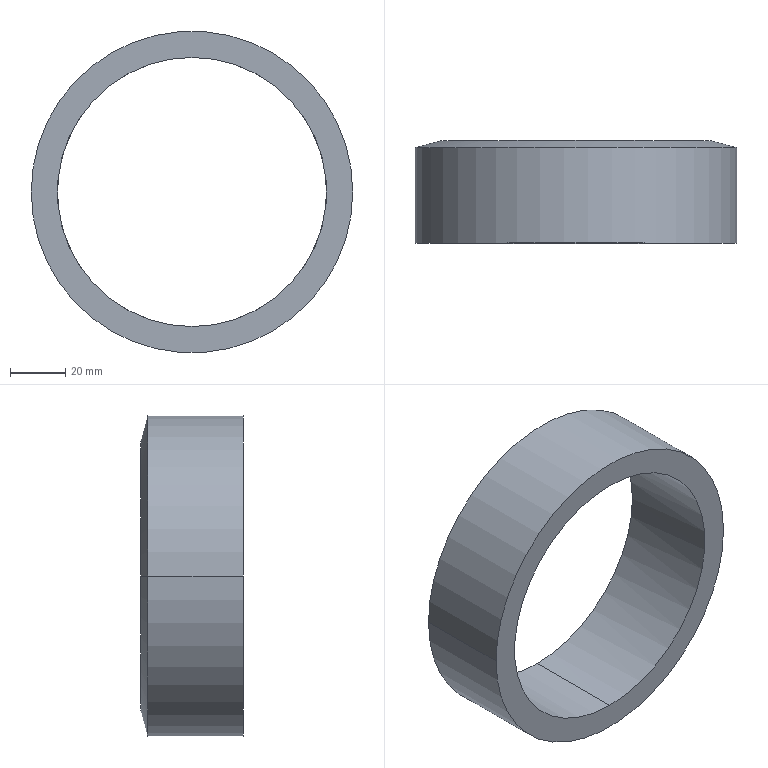Part | SolidWorks | features BaseBody 1 | 1 solid | 7 faces | box 116.16 x 37.047 x 116.16 mm | volume 113550 mm3 | cylinder 4 | cone 2 | plane 1 | commonest cylinder face diameters 97.2 x2 116.16 x2
STEP:
#1=CARTESIAN_POINT('',(-2181.55,1307.711,-1577.624));
#2=VERTEX_POINT('',#1);
#3=CARTESIAN_POINT('',(-2132.95,1307.711,-1626.224));
#4=VERTEX_POINT('',#3);
#5=CARTESIAN_POINT('',(-2132.95,1307.711,-1577.624));
#6=DIRECTION('',(0.,-1.,0.));
#7=DIRECTION('',(-1.,0.,0.));
#8=AXIS2_PLACEMENT_3D('',#5,#6,#7);
#9=CIRCLE('',#8,48.6);
#10=EDGE_CURVE('',#2,#4,#9,.T.);
#11=ORIENTED_EDGE('',*,*,#10,.F.);
#12=CARTESIAN_POINT('',(-2132.95,1307.711,-1529.024));
#13=VERTEX_POINT('',#12);
#14=CARTESIAN_POINT('',(-2132.95,1307.711,-1577.624));
#15=DIRECTION('',(0.,-1.,0.));
#16=DIRECTION('',(0.,0.,1.));
#17=AXIS2_PLACEMENT_3D('',#14,#15,#16);
#18=CIRCLE('',#17,48.6);
#19=EDGE_CURVE('',#13,#2,#18,.T.);
#20=ORIENTED_EDGE('',*,*,#19,.F.);
#21=CARTESIAN_POINT('',(-2132.95,1270.664,-1529.024));
#22=VERTEX_POINT('',#21);
#23=CARTESIAN_POINT('',(-2132.95,1307.711,-1529.024));
#24=DIRECTION('',(0.,-1.,0.));
#25=VECTOR('',#24,1000.);
#26=LINE('',#23,#25);
#27=EDGE_CURVE('',#13,#22,#26,.T.);
#28=ORIENTED_EDGE('',*,*,#27,.T.);
#29=CARTESIAN_POINT('',(-2132.95,1270.664,-1626.224));
#30=VERTEX_POINT('',#29);
#31=CARTESIAN_POINT('',(-2132.95,1270.664,-1577.624));
#32=DIRECTION('',(0.,-1.,0.));
#33=DIRECTION('',(0.,0.,1.));
#34=AXIS2_PLACEMENT_3D('',#31,#32,#33);
#35=CIRCLE('',#34,48.6);
#36=EDGE_CURVE('',#22,#30,#35,.T.);
#37=ORIENTED_EDGE('',*,*,#36,.T.);
#38=CARTESIAN_POINT('',(-2132.95,1307.711,-1626.224));
#39=DIRECTION('',(0.,-1.,0.));
#40=VECTOR('',#39,1000.);
#41=LINE('',#38,#40);
#42=EDGE_CURVE('',#4,#30,#41,.T.);
#43=ORIENTED_EDGE('',*,*,#42,.F.);
#44=EDGE_LOOP('',(#11,#20,#28,#37,#43));
#45=FACE_OUTER_BOUND('',#44,.T.);
#46=CARTESIAN_POINT('',(-2132.95,1309.563,-1577.624));
#47=DIRECTION('',(0.,-1.,0.));
#48=DIRECTION('',(0.08716,0.,0.9962));
#49=AXIS2_PLACEMENT_3D('',#46,#47,#48);
#50=CYLINDRICAL_SURFACE('',#49,48.6);
#51=ADVANCED_FACE('',(#45),#50,.F.);
#52=CARTESIAN_POINT('',(-2084.35,1307.711,-1577.624));
#53=VERTEX_POINT('',#52);
#54=CARTESIAN_POINT('',(-2132.95,1307.711,-1577.624));
#55=DIRECTION('',(0.,-1.,0.));
#56=DIRECTION('',(1.,0.,0.));
#57=AXIS2_PLACEMENT_3D('',#54,#55,#56);
#58=CIRCLE('',#57,48.6);
#59=EDGE_CURVE('',#53,#13,#58,.T.);
#60=ORIENTED_EDGE('',*,*,#59,.F.);
#61=CARTESIAN_POINT('',(-2132.95,1307.711,-1577.624));
#62=DIRECTION('',(0.,-1.,0.));
#63=DIRECTION('',(0.,0.,-1.));
#64=AXIS2_PLACEMENT_3D('',#61,#62,#63);
#65=CIRCLE('',#64,48.6);
#66=EDGE_CURVE('',#4,#53,#65,.T.);
#67=ORIENTED_EDGE('',*,*,#66,.F.);
#68=ORIENTED_EDGE('',*,*,#42,.T.);
#69=CARTESIAN_POINT('',(-2132.95,1270.664,-1577.624));
#70=DIRECTION('',(0.,-1.,0.));
#71=DIRECTION('',(0.,0.,-1.));
#72=AXIS2_PLACEMENT_3D('',#69,#70,#71);
#73=CIRCLE('',#72,48.6);
#74=EDGE_CURVE('',#30,#22,#73,.T.);
#75=ORIENTED_EDGE('',*,*,#74,.T.);
#76=ORIENTED_EDGE('',*,*,#27,.F.);
#77=EDGE_LOOP('',(#60,#67,#68,#75,#76));
#78=FACE_OUTER_BOUND('',#77,.T.);
#79=CARTESIAN_POINT('',(-2132.95,1309.563,-1577.624));
#80=DIRECTION('',(0.,-1.,0.));
#81=DIRECTION('',(-0.08716,0.,-0.9962));
#82=AXIS2_PLACEMENT_3D('',#79,#80,#81);
#83=CYLINDRICAL_SURFACE('',#82,48.6);
#84=ADVANCED_FACE('',(#78),#83,.F.);
#85=CARTESIAN_POINT('',(-2074.87,1305.171,-1577.624));
#86=VERTEX_POINT('',#85);
#87=CARTESIAN_POINT('',(-2084.35,1307.711,-1577.624));
#88=DIRECTION('',(0.9659,-0.2588,0.));
#89=VECTOR('',#88,1000.);
#90=LINE('',#87,#89);
#91=EDGE_CURVE('',#53,#86,#90,.T.);
#92=ORIENTED_EDGE('',*,*,#91,.F.);
#93=ORIENTED_EDGE('',*,*,#59,.T.);
#94=ORIENTED_EDGE('',*,*,#19,.T.);
#95=CARTESIAN_POINT('',(-2191.03,1305.171,-1577.624));
#96=VERTEX_POINT('',#95);
#97=CARTESIAN_POINT('',(-2181.55,1307.711,-1577.624));
#98=DIRECTION('',(-0.9659,-0.2588,0.));
#99=VECTOR('',#98,1000.);
#100=LINE('',#97,#99);
#101=EDGE_CURVE('',#2,#96,#100,.T.);
#102=ORIENTED_EDGE('',*,*,#101,.T.);
#103=CARTESIAN_POINT('',(-2132.95,1305.171,-1577.624));
#104=DIRECTION('',(0.,1.,0.));
#105=DIRECTION('',(-1.,0.,0.));
#106=AXIS2_PLACEMENT_3D('',#103,#104,#105);
#107=CIRCLE('',#106,58.08);
#108=EDGE_CURVE('',#96,#86,#107,.T.);
#109=ORIENTED_EDGE('',*,*,#108,.T.);
#110=EDGE_LOOP('',(#92,#93,#94,#102,#109));
#111=FACE_OUTER_BOUND('',#110,.T.);
#112=CARTESIAN_POINT('',(-2132.95,1307.838,-1577.624));
#113=DIRECTION('',(0.,-1.,0.));
#114=DIRECTION('',(0.9962,0.,-0.08716));
#115=AXIS2_PLACEMENT_3D('',#112,#113,#114);
#116=CONICAL_SURFACE('',#115,48.126,1.309);
#117=ADVANCED_FACE('',(#111),#116,.T.);
#118=ORIENTED_EDGE('',*,*,#108,.F.);
#119=CARTESIAN_POINT('',(-2191.03,1270.664,-1577.624));
#120=VERTEX_POINT('',#119);
#121=CARTESIAN_POINT('',(-2191.03,1305.171,-1577.624));
#122=DIRECTION('',(0.,-1.,0.));
#123=VECTOR('',#122,1000.);
#124=LINE('',#121,#123);
#125=EDGE_CURVE('',#96,#120,#124,.T.);
#126=ORIENTED_EDGE('',*,*,#125,.T.);
#127=CARTESIAN_POINT('',(-2074.87,1270.664,-1577.624));
#128=VERTEX_POINT('',#127);
#129=CARTESIAN_POINT('',(-2132.95,1270.664,-1577.624));
#130=DIRECTION('',(0.,-1.,0.));
#131=DIRECTION('',(1.,0.,0.));
#132=AXIS2_PLACEMENT_3D('',#129,#130,#131);
#133=CIRCLE('',#132,58.08);
#134=EDGE_CURVE('',#128,#120,#133,.T.);
#135=ORIENTED_EDGE('',*,*,#134,.F.);
#136=CARTESIAN_POINT('',(-2074.87,1305.171,-1577.624));
#137=DIRECTION('',(0.,-1.,0.));
#138=VECTOR('',#137,1000.);
#139=LINE('',#136,#138);
#140=EDGE_CURVE('',#86,#128,#139,.T.);
#141=ORIENTED_EDGE('',*,*,#140,.F.);
#142=EDGE_LOOP('',(#118,#126,#135,#141));
#143=FACE_OUTER_BOUND('',#142,.T.);
#144=CARTESIAN_POINT('',(-2132.95,1268.939,-1577.624));
#145=DIRECTION('',(0.,-1.,0.));
#146=DIRECTION('',(0.9962,0.,-0.08716));
#147=AXIS2_PLACEMENT_3D('',#144,#145,#146);
#148=CYLINDRICAL_SURFACE('',#147,58.08);
#149=ADVANCED_FACE('',(#143),#148,.T.);
#150=ORIENTED_EDGE('',*,*,#125,.F.);
#151=CARTESIAN_POINT('',(-2132.95,1305.171,-1577.624));
#152=DIRECTION('',(0.,1.,0.));
#153=DIRECTION('',(1.,0.,0.));
#154=AXIS2_PLACEMENT_3D('',#151,#152,#153);
#155=CIRCLE('',#154,58.08);
#156=EDGE_CURVE('',#86,#96,#155,.T.);
#157=ORIENTED_EDGE('',*,*,#156,.F.);
#158=ORIENTED_EDGE('',*,*,#140,.T.);
#159=CARTESIAN_POINT('',(-2132.95,1270.664,-1577.624));
#160=DIRECTION('',(0.,-1.,0.));
#161=DIRECTION('',(-1.,0.,0.));
#162=AXIS2_PLACEMENT_3D('',#159,#160,#161);
#163=CIRCLE('',#162,58.08);
#164=EDGE_CURVE('',#120,#128,#163,.T.);
#165=ORIENTED_EDGE('',*,*,#164,.F.);
#166=EDGE_LOOP('',(#150,#157,#158,#165));
#167=FACE_OUTER_BOUND('',#166,.T.);
#168=CARTESIAN_POINT('',(-2132.95,1268.939,-1577.624));
#169=DIRECTION('',(0.,-1.,0.));
#170=DIRECTION('',(-0.9962,0.,0.08716));
#171=AXIS2_PLACEMENT_3D('',#168,#169,#170);
#172=CYLINDRICAL_SURFACE('',#171,58.08);
#173=ADVANCED_FACE('',(#167),#172,.T.);
#174=ORIENTED_EDGE('',*,*,#74,.F.);
#175=ORIENTED_EDGE('',*,*,#36,.F.);
#176=EDGE_LOOP('',(#174,#175));
#177=FACE_BOUND('',#176,.T.);
#178=ORIENTED_EDGE('',*,*,#164,.T.);
#179=ORIENTED_EDGE('',*,*,#134,.T.);
#180=EDGE_LOOP('',(#178,#179));
#181=FACE_OUTER_BOUND('',#180,.T.);
#182=CARTESIAN_POINT('',(-2069.062,1270.664,-1513.752));
#183=DIRECTION('',(0.,-1.,0.));
#184=DIRECTION('',(0.,0.,-1.));
#185=AXIS2_PLACEMENT_3D('',#182,#183,#184);
#186=PLANE('',#185);
#187=ADVANCED_FACE('',(#177,#181),#186,.T.);
#188=ORIENTED_EDGE('',*,*,#101,.F.);
#189=ORIENTED_EDGE('',*,*,#10,.T.);
#190=ORIENTED_EDGE('',*,*,#66,.T.);
#191=ORIENTED_EDGE('',*,*,#91,.T.);
#192=ORIENTED_EDGE('',*,*,#156,.T.);
#193=EDGE_LOOP('',(#188,#189,#190,#191,#192));
#194=FACE_OUTER_BOUND('',#193,.T.);
#195=CARTESIAN_POINT('',(-2132.95,1307.838,-1577.624));
#196=DIRECTION('',(0.,-1.,0.));
#197=DIRECTION('',(-0.9962,0.,0.08716));
#198=AXIS2_PLACEMENT_3D('',#195,#196,#197);
#199=CONICAL_SURFACE('',#198,48.126,1.309);
#200=ADVANCED_FACE('',(#194),#199,.T.);
#201=CLOSED_SHELL('',(#51,#84,#117,#149,#173,#187,#200));
#202=MANIFOLD_SOLID_BREP('',#201);
#203=CARTESIAN_POINT('',(0.,0.,0.));
#204=DIRECTION('',(0.,0.,1.));
#205=DIRECTION('',(1.,0.,0.));
#206=AXIS2_PLACEMENT_3D('',#203,#204,#205);
#207=(LENGTH_UNIT()NAMED_UNIT(*)SI_UNIT(.MILLI.,.METRE.));
#208=UNCERTAINTY_MEASURE_WITH_UNIT(LENGTH_MEASURE(0.00001),#207,'','');
#209=(NAMED_UNIT(*)PLANE_ANGLE_UNIT()SI_UNIT($,.RADIAN.));
#210=(NAMED_UNIT(*)SI_UNIT($,.STERADIAN.)SOLID_ANGLE_UNIT());
#211=(GEOMETRIC_REPRESENTATION_CONTEXT(3)GLOBAL_UNCERTAINTY_ASSIGNED_CONTEXT((#208))GLOBAL_UNIT_ASSIGNED_CONTEXT((#207,#209,#210))REPRESENTATION_CONTEXT('',''));
#212=ADVANCED_BREP_SHAPE_REPRESENTATION('',(#202,#206),#211);